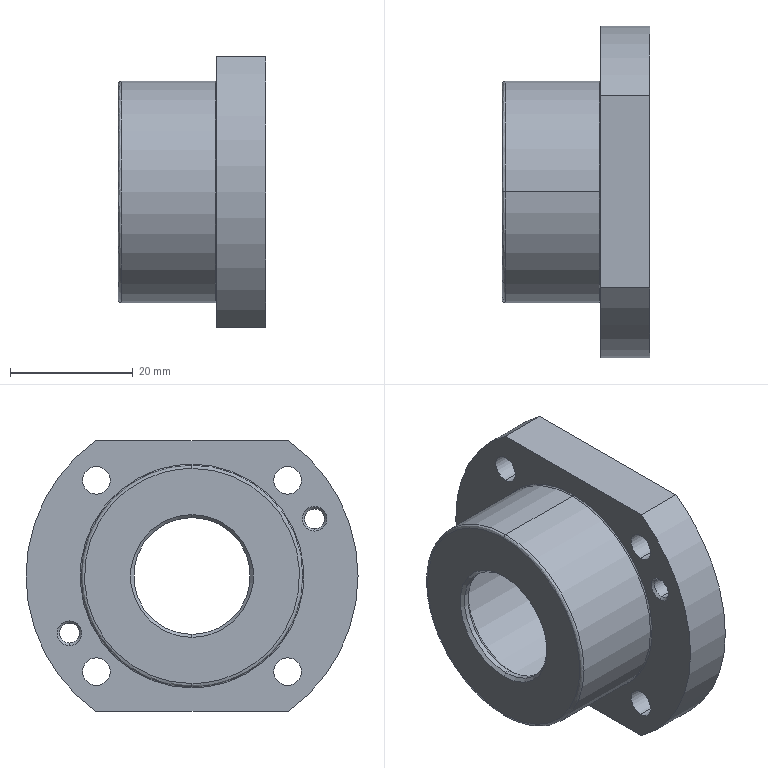Part | SolidWorks | features BaseBody 1 | 1 solid | 64 faces | box 24 x 54 x 44 mm | volume 16964 mm3 | cylinder 32 | cone 14 | plane 12 | spline 6 | commonest cylinder face diameters 4.5 x8 8 x8 3.242 x4 19 x2 28 x2 30 x2